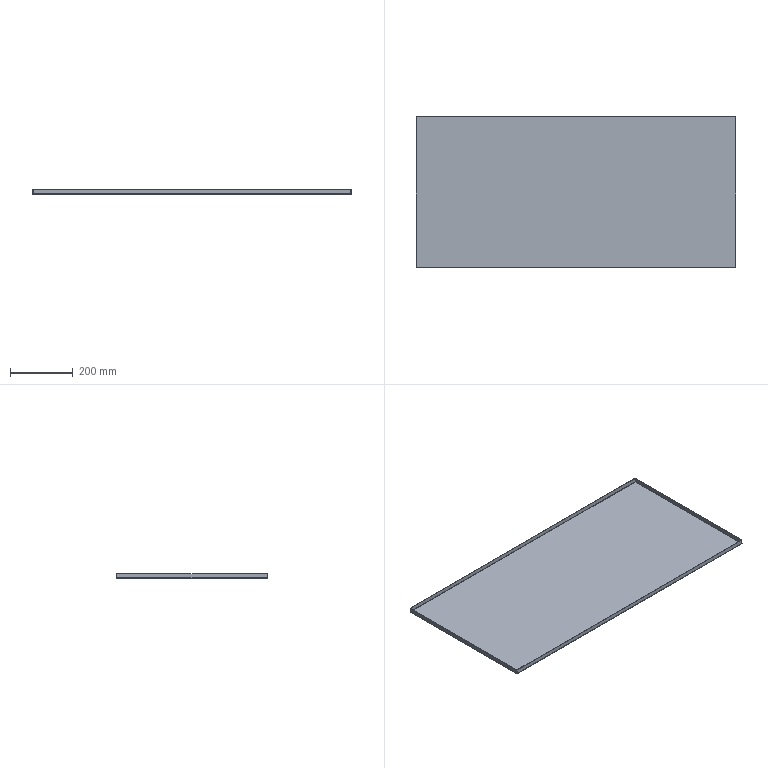Part | SolidWorks | 1 solid | 38 faces | box 1020 x 485.001 x 15 mm | volume 800985 mm3 | plane 22 | spline 8 | cylinder 8 | commonest cylinder face diameters 0.2 x4 3.2 x4
STEP:
#1=CARTESIAN_POINT('',(508.4,-240.9,-1.5));
#2=VERTEX_POINT('',#1);
#3=CARTESIAN_POINT('',(-508.4,-240.9,-1.5));
#4=VERTEX_POINT('',#3);
#5=CARTESIAN_POINT('',(508.4,-240.9,-1.5));
#6=DIRECTION('',(-1.,0.,0.));
#7=VECTOR('',#6,1000.);
#8=LINE('',#5,#7);
#9=EDGE_CURVE('',#2,#4,#8,.T.);
#10=ORIENTED_EDGE('',*,*,#9,.T.);
#11=CARTESIAN_POINT('',(-508.4,240.9,-1.5));
#12=VERTEX_POINT('',#11);
#13=CARTESIAN_POINT('',(-508.4,-240.9,-1.5));
#14=DIRECTION('',(0.,1.,0.));
#15=VECTOR('',#14,1000.);
#16=LINE('',#13,#15);
#17=EDGE_CURVE('',#4,#12,#16,.T.);
#18=ORIENTED_EDGE('',*,*,#17,.T.);
#19=CARTESIAN_POINT('',(508.4,240.9,-1.5));
#20=VERTEX_POINT('',#19);
#21=CARTESIAN_POINT('',(-508.4,240.9,-1.5));
#22=DIRECTION('',(1.,0.,0.));
#23=VECTOR('',#22,1000.);
#24=LINE('',#21,#23);
#25=EDGE_CURVE('',#12,#20,#24,.T.);
#26=ORIENTED_EDGE('',*,*,#25,.T.);
#27=CARTESIAN_POINT('',(508.4,240.9,-1.5));
#28=DIRECTION('',(0.,-1.,0.));
#29=VECTOR('',#28,1000.);
#30=LINE('',#27,#29);
#31=EDGE_CURVE('',#20,#2,#30,.T.);
#32=ORIENTED_EDGE('',*,*,#31,.T.);
#33=EDGE_LOOP('',(#10,#18,#26,#32));
#34=FACE_OUTER_BOUND('',#33,.T.);
#35=CARTESIAN_POINT('',(0.,0.,-1.5));
#36=DIRECTION('',(0.,0.,1.));
#37=DIRECTION('',(1.,0.,0.));
#38=AXIS2_PLACEMENT_3D('',#35,#36,#37);
#39=PLANE('',#38);
#40=ADVANCED_FACE('',(#34),#39,.F.);
#41=CARTESIAN_POINT('',(-508.4,-240.9,0.));
#42=VERTEX_POINT('',#41);
#43=CARTESIAN_POINT('',(-508.4,240.9,0.));
#44=VERTEX_POINT('',#43);
#45=CARTESIAN_POINT('',(-508.4,-240.9,0.));
#46=DIRECTION('',(0.,1.,0.));
#47=VECTOR('',#46,1000.);
#48=LINE('',#45,#47);
#49=EDGE_CURVE('',#42,#44,#48,.T.);
#50=ORIENTED_EDGE('',*,*,#49,.F.);
#51=CARTESIAN_POINT('',(508.4,-240.9,0.));
#52=VERTEX_POINT('',#51);
#53=CARTESIAN_POINT('',(508.4,-240.9,0.));
#54=DIRECTION('',(-1.,0.,0.));
#55=VECTOR('',#54,1000.);
#56=LINE('',#53,#55);
#57=EDGE_CURVE('',#52,#42,#56,.T.);
#58=ORIENTED_EDGE('',*,*,#57,.F.);
#59=CARTESIAN_POINT('',(508.4,240.9,0.));
#60=VERTEX_POINT('',#59);
#61=CARTESIAN_POINT('',(508.4,240.9,0.));
#62=DIRECTION('',(0.,-1.,0.));
#63=VECTOR('',#62,1000.);
#64=LINE('',#61,#63);
#65=EDGE_CURVE('',#60,#52,#64,.T.);
#66=ORIENTED_EDGE('',*,*,#65,.F.);
#67=CARTESIAN_POINT('',(-508.4,240.9,0.));
#68=DIRECTION('',(1.,0.,0.));
#69=VECTOR('',#68,1000.);
#70=LINE('',#67,#69);
#71=EDGE_CURVE('',#44,#60,#70,.T.);
#72=ORIENTED_EDGE('',*,*,#71,.F.);
#73=EDGE_LOOP('',(#50,#58,#66,#72));
#74=FACE_OUTER_BOUND('',#73,.T.);
#75=CARTESIAN_POINT('',(0.,0.,0.));
#76=DIRECTION('',(0.,0.,1.));
#77=DIRECTION('',(1.,0.,0.));
#78=AXIS2_PLACEMENT_3D('',#75,#76,#77);
#79=PLANE('',#78);
#80=ADVANCED_FACE('',(#74),#79,.T.);
#81=CARTESIAN_POINT('',(-510.,240.293,0.1));
#82=VERTEX_POINT('',#81);
#83=CARTESIAN_POINT('',(-508.5,240.293,0.1));
#84=VERTEX_POINT('',#83);
#85=CARTESIAN_POINT('',(-508.5,240.293,0.1));
#86=DIRECTION('',(1.,0.,0.));
#87=VECTOR('',#86,1000.);
#88=LINE('',#85,#87);
#89=EDGE_CURVE('',#82,#84,#88,.T.);
#90=ORIENTED_EDGE('',*,*,#89,.T.);
#91=CARTESIAN_POINT('',(-508.4,240.9,0.));
#92=CARTESIAN_POINT('',(-508.426,240.799,0.));
#93=CARTESIAN_POINT('',(-508.452,240.698,0.01078));
#94=CARTESIAN_POINT('',(-508.489,240.495,0.0478));
#95=CARTESIAN_POINT('',(-508.5,240.394,0.07382));
#96=CARTESIAN_POINT('',(-508.5,240.293,0.1));
#97=B_SPLINE_CURVE_WITH_KNOTS('',3,(#91,#92,#93,#94,#95,#96),.UNSPECIFIED.,.F.,.F.,(4,2,4),(0.,0.5,1.),.UNSPECIFIED.);
#98=EDGE_CURVE('',#44,#84,#97,.T.);
#99=ORIENTED_EDGE('',*,*,#98,.F.);
#100=CARTESIAN_POINT('',(-508.4,240.9,0.));
#101=DIRECTION('',(0.,0.,-1.));
#102=VECTOR('',#101,1000.);
#103=LINE('',#100,#102);
#104=EDGE_CURVE('',#44,#12,#103,.T.);
#105=ORIENTED_EDGE('',*,*,#104,.T.);
#106=CARTESIAN_POINT('',(-508.4,240.9,-1.5));
#107=CARTESIAN_POINT('',(-508.612,240.849,-1.5));
#108=CARTESIAN_POINT('',(-508.815,240.8,-1.46));
#109=CARTESIAN_POINT('',(-509.205,240.698,-1.299));
#110=CARTESIAN_POINT('',(-509.381,240.648,-1.181));
#111=CARTESIAN_POINT('',(-509.605,240.571,-0.9582));
#112=CARTESIAN_POINT('',(-509.671,240.546,-0.8775));
#113=CARTESIAN_POINT('',(-509.787,240.496,-0.7041));
#114=CARTESIAN_POINT('',(-509.838,240.47,-0.6103));
#115=CARTESIAN_POINT('',(-509.958,240.394,-0.32));
#116=CARTESIAN_POINT('',(-510.,240.344,-0.1115));
#117=CARTESIAN_POINT('',(-510.,240.293,0.1));
#118=B_SPLINE_CURVE_WITH_KNOTS('',3,(#106,#107,#108,#109,#110,#111,#112,#113,#114,#115,#116,#117),.UNSPECIFIED.,.F.,.F.,(4,2,2,2,2,4),(0.,0.0006399,0.00128,0.0016,0.00192,0.00256),.UNSPECIFIED.);
#119=EDGE_CURVE('',#12,#82,#118,.T.);
#120=ORIENTED_EDGE('',*,*,#119,.T.);
#121=EDGE_LOOP('',(#90,#99,#105,#120));
#122=FACE_OUTER_BOUND('',#121,.T.);
#123=CARTESIAN_POINT('',(-508.4,240.9,-1.515));
#124=CARTESIAN_POINT('',(-508.611,240.849,-1.515));
#125=CARTESIAN_POINT('',(-508.823,240.799,-1.473));
#126=CARTESIAN_POINT('',(-509.213,240.698,-1.311));
#127=CARTESIAN_POINT('',(-509.392,240.647,-1.191));
#128=CARTESIAN_POINT('',(-509.691,240.546,-0.8925));
#129=CARTESIAN_POINT('',(-509.811,240.495,-0.7133));
#130=CARTESIAN_POINT('',(-509.973,240.394,-0.3227));
#131=CARTESIAN_POINT('',(-510.015,240.343,-0.1114));
#132=CARTESIAN_POINT('',(-510.015,240.293,0.1));
#133=CARTESIAN_POINT('',(-508.4,240.9,-1.5));
#134=CARTESIAN_POINT('',(-508.609,240.849,-1.5));
#135=CARTESIAN_POINT('',(-508.819,240.799,-1.458));
#136=CARTESIAN_POINT('',(-509.206,240.698,-1.298));
#137=CARTESIAN_POINT('',(-509.383,240.647,-1.179));
#138=CARTESIAN_POINT('',(-509.679,240.546,-0.8833));
#139=CARTESIAN_POINT('',(-509.798,240.495,-0.7058));
#140=CARTESIAN_POINT('',(-509.958,240.394,-0.3188));
#141=CARTESIAN_POINT('',(-510.,240.343,-0.1095));
#142=CARTESIAN_POINT('',(-510.,240.293,0.1));
#143=CARTESIAN_POINT('',(-508.4,240.9,0.));
#144=CARTESIAN_POINT('',(-508.413,240.849,0.));
#145=CARTESIAN_POINT('',(-508.426,240.799,0.002603));
#146=CARTESIAN_POINT('',(-508.45,240.698,0.01262));
#147=CARTESIAN_POINT('',(-508.461,240.647,0.02003));
#148=CARTESIAN_POINT('',(-508.48,240.546,0.03855));
#149=CARTESIAN_POINT('',(-508.487,240.495,0.04964));
#150=CARTESIAN_POINT('',(-508.497,240.394,0.07383));
#151=CARTESIAN_POINT('',(-508.5,240.343,0.08691));
#152=CARTESIAN_POINT('',(-508.5,240.293,0.1));
#153=B_SPLINE_SURFACE_WITH_KNOTS('',1,3,((#123,#124,#125,#126,#127,#128,#129,#130,#131,#132),(#133,#134,#135,#136,#137,#138,#139,#140,#141,#142),(#143,#144,#145,#146,#147,#148,#149,#150,#151,#152)),.UNSPECIFIED.,.F.,.F.,.F.,(2,1,2),(4,2,2,2,4),(-0.01,0.,1.),(0.,0.25,0.5,0.75,1.),.UNSPECIFIED.);
#154=ADVANCED_FACE('',(#122),#153,.F.);
#155=CARTESIAN_POINT('',(-508.5,-240.293,0.1));
#156=VERTEX_POINT('',#155);
#157=CARTESIAN_POINT('',(-508.5,-240.293,0.1));
#158=CARTESIAN_POINT('',(-508.5,-240.394,0.07382));
#159=CARTESIAN_POINT('',(-508.489,-240.495,0.0478));
#160=CARTESIAN_POINT('',(-508.452,-240.698,0.01078));
#161=CARTESIAN_POINT('',(-508.426,-240.799,0.));
#162=CARTESIAN_POINT('',(-508.4,-240.9,0.));
#163=B_SPLINE_CURVE_WITH_KNOTS('',3,(#157,#158,#159,#160,#161,#162),.UNSPECIFIED.,.F.,.F.,(4,2,4),(0.,0.5,1.),.UNSPECIFIED.);
#164=EDGE_CURVE('',#156,#42,#163,.T.);
#165=ORIENTED_EDGE('',*,*,#164,.F.);
#166=CARTESIAN_POINT('',(-510.,-240.293,0.1));
#167=VERTEX_POINT('',#166);
#168=CARTESIAN_POINT('',(-508.5,-240.293,0.1));
#169=DIRECTION('',(1.,0.,0.));
#170=VECTOR('',#169,1000.);
#171=LINE('',#168,#170);
#172=EDGE_CURVE('',#167,#156,#171,.T.);
#173=ORIENTED_EDGE('',*,*,#172,.F.);
#174=CARTESIAN_POINT('',(-510.,-240.293,0.1));
#175=CARTESIAN_POINT('',(-510.,-240.344,-0.1115));
#176=CARTESIAN_POINT('',(-509.96,-240.393,-0.3151));
#177=CARTESIAN_POINT('',(-509.799,-240.495,-0.7048));
#178=CARTESIAN_POINT('',(-509.681,-240.545,-0.881));
#179=CARTESIAN_POINT('',(-509.458,-240.621,-1.105));
#180=CARTESIAN_POINT('',(-509.378,-240.647,-1.171));
#181=CARTESIAN_POINT('',(-509.204,-240.697,-1.287));
#182=CARTESIAN_POINT('',(-509.11,-240.723,-1.338));
#183=CARTESIAN_POINT('',(-508.82,-240.799,-1.458));
#184=CARTESIAN_POINT('',(-508.612,-240.849,-1.5));
#185=CARTESIAN_POINT('',(-508.4,-240.9,-1.5));
#186=B_SPLINE_CURVE_WITH_KNOTS('',3,(#174,#175,#176,#177,#178,#179,#180,#181,#182,#183,#184,#185),.UNSPECIFIED.,.F.,.F.,(4,2,2,2,2,4),(0.,0.0006399,0.00128,0.0016,0.00192,0.00256),.UNSPECIFIED.);
#187=EDGE_CURVE('',#167,#4,#186,.T.);
#188=ORIENTED_EDGE('',*,*,#187,.T.);
#189=CARTESIAN_POINT('',(-508.4,-240.9,0.));
#190=DIRECTION('',(0.,0.,-1.));
#191=VECTOR('',#190,1000.);
#192=LINE('',#189,#191);
#193=EDGE_CURVE('',#42,#4,#192,.T.);
#194=ORIENTED_EDGE('',*,*,#193,.F.);
#195=EDGE_LOOP('',(#165,#173,#188,#194));
#196=FACE_OUTER_BOUND('',#195,.T.);
#197=CARTESIAN_POINT('',(-510.015,-240.293,0.1));
#198=CARTESIAN_POINT('',(-510.015,-240.343,-0.1114));
#199=CARTESIAN_POINT('',(-509.973,-240.394,-0.3227));
#200=CARTESIAN_POINT('',(-509.811,-240.495,-0.7133));
#201=CARTESIAN_POINT('',(-509.691,-240.546,-0.8925));
#202=CARTESIAN_POINT('',(-509.392,-240.647,-1.191));
#203=CARTESIAN_POINT('',(-509.213,-240.698,-1.311));
#204=CARTESIAN_POINT('',(-508.823,-240.799,-1.473));
#205=CARTESIAN_POINT('',(-508.611,-240.849,-1.515));
#206=CARTESIAN_POINT('',(-508.4,-240.9,-1.515));
#207=CARTESIAN_POINT('',(-510.,-240.293,0.1));
#208=CARTESIAN_POINT('',(-510.,-240.343,-0.1095));
#209=CARTESIAN_POINT('',(-509.958,-240.394,-0.3188));
#210=CARTESIAN_POINT('',(-509.798,-240.495,-0.7058));
#211=CARTESIAN_POINT('',(-509.679,-240.546,-0.8833));
#212=CARTESIAN_POINT('',(-509.383,-240.647,-1.179));
#213=CARTESIAN_POINT('',(-509.206,-240.698,-1.298));
#214=CARTESIAN_POINT('',(-508.819,-240.799,-1.458));
#215=CARTESIAN_POINT('',(-508.609,-240.849,-1.5));
#216=CARTESIAN_POINT('',(-508.4,-240.9,-1.5));
#217=CARTESIAN_POINT('',(-508.5,-240.293,0.1));
#218=CARTESIAN_POINT('',(-508.5,-240.343,0.08691));
#219=CARTESIAN_POINT('',(-508.497,-240.394,0.07383));
#220=CARTESIAN_POINT('',(-508.487,-240.495,0.04964));
#221=CARTESIAN_POINT('',(-508.48,-240.546,0.03855));
#222=CARTESIAN_POINT('',(-508.461,-240.647,0.02003));
#223=CARTESIAN_POINT('',(-508.45,-240.698,0.01262));
#224=CARTESIAN_POINT('',(-508.426,-240.799,0.002603));
#225=CARTESIAN_POINT('',(-508.413,-240.849,0.));
#226=CARTESIAN_POINT('',(-508.4,-240.9,0.));
#227=B_SPLINE_SURFACE_WITH_KNOTS('',1,3,((#197,#198,#199,#200,#201,#202,#203,#204,#205,#206),(#207,#208,#209,#210,#211,#212,#213,#214,#215,#216),(#217,#218,#219,#220,#221,#222,#223,#224,#225,#226)),.UNSPECIFIED.,.F.,.F.,.F.,(2,1,2),(4,2,2,2,4),(-0.01,0.,1.),(0.,0.25,0.5,0.75,1.),.UNSPECIFIED.);
#228=ADVANCED_FACE('',(#196),#227,.F.);
#229=ORIENTED_EDGE('',*,*,#17,.F.);
#230=ORIENTED_EDGE('',*,*,#187,.F.);
#231=CARTESIAN_POINT('',(-510.,242.5,0.1));
#232=DIRECTION('',(0.,1.,0.));
#233=VECTOR('',#232,1000.);
#234=LINE('',#231,#233);
#235=EDGE_CURVE('',#167,#82,#234,.T.);
#236=ORIENTED_EDGE('',*,*,#235,.T.);
#237=ORIENTED_EDGE('',*,*,#119,.F.);
#238=EDGE_LOOP('',(#229,#230,#236,#237));
#239=FACE_OUTER_BOUND('',#238,.T.);
#240=CARTESIAN_POINT('',(-508.4,-240.9,0.1));
#241=DIRECTION('',(0.,-1.,0.));
#242=DIRECTION('',(-1.,0.,0.));
#243=AXIS2_PLACEMENT_3D('',#240,#241,#242);
#244=CYLINDRICAL_SURFACE('',#243,1.6);
#245=ADVANCED_FACE('',(#239),#244,.T.);
#246=ORIENTED_EDGE('',*,*,#49,.T.);
#247=ORIENTED_EDGE('',*,*,#98,.T.);
#248=CARTESIAN_POINT('',(-508.5,242.5,0.1));
#249=DIRECTION('',(0.,-1.,0.));
#250=VECTOR('',#249,1000.);
#251=LINE('',#248,#250);
#252=EDGE_CURVE('',#84,#156,#251,.T.);
#253=ORIENTED_EDGE('',*,*,#252,.T.);
#254=ORIENTED_EDGE('',*,*,#164,.T.);
#255=EDGE_LOOP('',(#246,#247,#253,#254));
#256=FACE_OUTER_BOUND('',#255,.T.);
#257=CARTESIAN_POINT('',(-508.4,-240.9,0.1));
#258=DIRECTION('',(0.,-1.,0.));
#259=DIRECTION('',(-1.,0.,0.));
#260=AXIS2_PLACEMENT_3D('',#257,#258,#259);
#261=CYLINDRICAL_SURFACE('',#260,0.1);
#262=ADVANCED_FACE('',(#256),#261,.F.);
#263=CARTESIAN_POINT('',(-510.,240.293,13.5));
#264=VERTEX_POINT('',#263);
#265=CARTESIAN_POINT('',(-510.,240.293,0.));
#266=DIRECTION('',(0.,0.,1.));
#267=VECTOR('',#266,1000.);
#268=LINE('',#265,#267);
#269=EDGE_CURVE('',#82,#264,#268,.T.);
#270=ORIENTED_EDGE('',*,*,#269,.T.);
#271=CARTESIAN_POINT('',(-508.5,240.293,13.5));
#272=VERTEX_POINT('',#271);
#273=CARTESIAN_POINT('',(-508.5,240.293,13.5));
#274=DIRECTION('',(1.,0.,0.));
#275=VECTOR('',#274,1000.);
#276=LINE('',#273,#275);
#277=EDGE_CURVE('',#264,#272,#276,.T.);
#278=ORIENTED_EDGE('',*,*,#277,.T.);
#279=CARTESIAN_POINT('',(-508.5,240.293,0.));
#280=DIRECTION('',(0.,0.,1.));
#281=VECTOR('',#280,1000.);
#282=LINE('',#279,#281);
#283=EDGE_CURVE('',#84,#272,#282,.T.);
#284=ORIENTED_EDGE('',*,*,#283,.F.);
#285=ORIENTED_EDGE('',*,*,#89,.F.);
#286=EDGE_LOOP('',(#270,#278,#284,#285));
#287=FACE_OUTER_BOUND('',#286,.T.);
#288=CARTESIAN_POINT('',(-508.5,240.293,0.));
#289=DIRECTION('',(0.,1.,0.));
#290=DIRECTION('',(0.,0.,1.));
#291=AXIS2_PLACEMENT_3D('',#288,#289,#290);
#292=PLANE('',#291);
#293=ADVANCED_FACE('',(#287),#292,.T.);
#294=ORIENTED_EDGE('',*,*,#235,.F.);
#295=CARTESIAN_POINT('',(-510.,-240.293,13.5));
#296=VERTEX_POINT('',#295);
#297=CARTESIAN_POINT('',(-510.,-240.293,0.));
#298=DIRECTION('',(0.,0.,1.));
#299=VECTOR('',#298,1000.);
#300=LINE('',#297,#299);
#301=EDGE_CURVE('',#167,#296,#300,.T.);
#302=ORIENTED_EDGE('',*,*,#301,.T.);
#303=CARTESIAN_POINT('',(-510.,0.,13.5));
#304=DIRECTION('',(0.,1.,0.));
#305=VECTOR('',#304,1000.);
#306=LINE('',#303,#305);
#307=EDGE_CURVE('',#296,#264,#306,.T.);
#308=ORIENTED_EDGE('',*,*,#307,.T.);
#309=ORIENTED_EDGE('',*,*,#269,.F.);
#310=EDGE_LOOP('',(#294,#302,#308,#309));
#311=FACE_OUTER_BOUND('',#310,.T.);
#312=CARTESIAN_POINT('',(-510.,0.,0.));
#313=DIRECTION('',(1.,0.,0.));
#314=DIRECTION('',(0.,0.,-1.));
#315=AXIS2_PLACEMENT_3D('',#312,#313,#314);
#316=PLANE('',#315);
#317=ADVANCED_FACE('',(#311),#316,.F.);
#318=CARTESIAN_POINT('',(-508.5,-240.293,13.5));
#319=VERTEX_POINT('',#318);
#320=CARTESIAN_POINT('',(-508.5,-240.293,0.));
#321=DIRECTION('',(0.,0.,1.));
#322=VECTOR('',#321,1000.);
#323=LINE('',#320,#322);
#324=EDGE_CURVE('',#156,#319,#323,.T.);
#325=ORIENTED_EDGE('',*,*,#324,.F.);
#326=ORIENTED_EDGE('',*,*,#252,.F.);
#327=ORIENTED_EDGE('',*,*,#283,.T.);
#328=CARTESIAN_POINT('',(-508.5,242.5,13.5));
#329=DIRECTION('',(0.,1.,0.));
#330=VECTOR('',#329,1000.);
#331=LINE('',#328,#330);
#332=EDGE_CURVE('',#319,#272,#331,.T.);
#333=ORIENTED_EDGE('',*,*,#332,.F.);
#334=EDGE_LOOP('',(#325,#326,#327,#333));
#335=FACE_OUTER_BOUND('',#334,.T.);
#336=CARTESIAN_POINT('',(-508.5,0.,0.));
#337=DIRECTION('',(1.,0.,0.));
#338=DIRECTION('',(0.,0.,-1.));
#339=AXIS2_PLACEMENT_3D('',#336,#337,#338);
#340=PLANE('',#339);
#341=ADVANCED_FACE('',(#335),#340,.T.);
#342=ORIENTED_EDGE('',*,*,#307,.F.);
#343=CARTESIAN_POINT('',(-510.,-240.293,13.5));
#344=DIRECTION('',(1.,0.,0.));
#345=VECTOR('',#344,1000.);
#346=LINE('',#343,#345);
#347=EDGE_CURVE('',#296,#319,#346,.T.);
#348=ORIENTED_EDGE('',*,*,#347,.T.);
#349=ORIENTED_EDGE('',*,*,#332,.T.);
#350=ORIENTED_EDGE('',*,*,#277,.F.);
#351=EDGE_LOOP('',(#342,#348,#349,#350));
#352=FACE_OUTER_BOUND('',#351,.T.);
#353=CARTESIAN_POINT('',(-510.,242.5,13.5));
#354=DIRECTION('',(0.,0.,-1.));
#355=DIRECTION('',(-1.,0.,0.));
#356=AXIS2_PLACEMENT_3D('',#353,#354,#355);
#357=PLANE('',#356);
#358=ADVANCED_FACE('',(#352),#357,.F.);
#359=ORIENTED_EDGE('',*,*,#347,.F.);
#360=ORIENTED_EDGE('',*,*,#301,.F.);
#361=ORIENTED_EDGE('',*,*,#172,.T.);
#362=ORIENTED_EDGE('',*,*,#324,.T.);
#363=EDGE_LOOP('',(#359,#360,#361,#362));
#364=FACE_OUTER_BOUND('',#363,.T.);
#365=CARTESIAN_POINT('',(-508.5,-240.293,0.));
#366=DIRECTION('',(0.,1.,0.));
#367=DIRECTION('',(0.,0.,1.));
#368=AXIS2_PLACEMENT_3D('',#365,#366,#367);
#369=PLANE('',#368);
#370=ADVANCED_FACE('',(#364),#369,.F.);
#371=CARTESIAN_POINT('',(507.793,242.5,0.1));
#372=VERTEX_POINT('',#371);
#373=CARTESIAN_POINT('',(507.793,241.,0.1));
#374=VERTEX_POINT('',#373);
#375=CARTESIAN_POINT('',(507.793,241.,0.1));
#376=DIRECTION('',(0.,-1.,0.));
#377=VECTOR('',#376,1000.);
#378=LINE('',#375,#377);
#379=EDGE_CURVE('',#372,#374,#378,.T.);
#380=ORIENTED_EDGE('',*,*,#379,.T.);
#381=CARTESIAN_POINT('',(508.4,240.9,0.));
#382=CARTESIAN_POINT('',(508.299,240.926,0.));
#383=CARTESIAN_POINT('',(508.198,240.952,0.01078));
#384=CARTESIAN_POINT('',(507.995,240.989,0.0478));
#385=CARTESIAN_POINT('',(507.894,241.,0.07382));
#386=CARTESIAN_POINT('',(507.793,241.,0.1));
#387=B_SPLINE_CURVE_WITH_KNOTS('',3,(#381,#382,#383,#384,#385,#386),.UNSPECIFIED.,.F.,.F.,(4,2,4),(0.,0.5,1.),.UNSPECIFIED.);
#388=EDGE_CURVE('',#60,#374,#387,.T.);
#389=ORIENTED_EDGE('',*,*,#388,.F.);
#390=CARTESIAN_POINT('',(508.4,240.9,0.));
#391=DIRECTION('',(0.,0.,-1.));
#392=VECTOR('',#391,1000.);
#393=LINE('',#390,#392);
#394=EDGE_CURVE('',#60,#20,#393,.T.);
#395=ORIENTED_EDGE('',*,*,#394,.T.);
#396=CARTESIAN_POINT('',(508.4,240.9,-1.5));
#397=CARTESIAN_POINT('',(508.349,241.112,-1.5));
#398=CARTESIAN_POINT('',(508.3,241.315,-1.46));
#399=CARTESIAN_POINT('',(508.198,241.705,-1.299));
#400=CARTESIAN_POINT('',(508.148,241.881,-1.181));
#401=CARTESIAN_POINT('',(508.071,242.105,-0.9582));
#402=CARTESIAN_POINT('',(508.046,242.171,-0.8775));
#403=CARTESIAN_POINT('',(507.996,242.287,-0.7041));
#404=CARTESIAN_POINT('',(507.97,242.338,-0.6103));
#405=CARTESIAN_POINT('',(507.894,242.458,-0.32));
#406=CARTESIAN_POINT('',(507.844,242.5,-0.1115));
#407=CARTESIAN_POINT('',(507.793,242.5,0.1));
#408=B_SPLINE_CURVE_WITH_KNOTS('',3,(#396,#397,#398,#399,#400,#401,#402,#403,#404,#405,#406,#407),.UNSPECIFIED.,.F.,.F.,(4,2,2,2,2,4),(0.,0.0006399,0.00128,0.0016,0.00192,0.00256),.UNSPECIFIED.);
#409=EDGE_CURVE('',#20,#372,#408,.T.);
#410=ORIENTED_EDGE('',*,*,#409,.T.);
#411=EDGE_LOOP('',(#380,#389,#395,#410));
#412=FACE_OUTER_BOUND('',#411,.T.);
#413=CARTESIAN_POINT('',(508.4,240.9,-1.515));
#414=CARTESIAN_POINT('',(508.349,241.111,-1.515));
#415=CARTESIAN_POINT('',(508.299,241.323,-1.473));
#416=CARTESIAN_POINT('',(508.198,241.713,-1.311));
#417=CARTESIAN_POINT('',(508.147,241.892,-1.191));
#418=CARTESIAN_POINT('',(508.046,242.191,-0.8925));
#419=CARTESIAN_POINT('',(507.995,242.311,-0.7133));
#420=CARTESIAN_POINT('',(507.894,242.473,-0.3227));
#421=CARTESIAN_POINT('',(507.843,242.515,-0.1114));
#422=CARTESIAN_POINT('',(507.793,242.515,0.1));
#423=CARTESIAN_POINT('',(508.4,240.9,-1.5));
#424=CARTESIAN_POINT('',(508.349,241.109,-1.5));
#425=CARTESIAN_POINT('',(508.299,241.319,-1.458));
#426=CARTESIAN_POINT('',(508.198,241.706,-1.298));
#427=CARTESIAN_POINT('',(508.147,241.883,-1.179));
#428=CARTESIAN_POINT('',(508.046,242.179,-0.8833));
#429=CARTESIAN_POINT('',(507.995,242.298,-0.7058));
#430=CARTESIAN_POINT('',(507.894,242.458,-0.3188));
#431=CARTESIAN_POINT('',(507.843,242.5,-0.1095));
#432=CARTESIAN_POINT('',(507.793,242.5,0.1));
#433=CARTESIAN_POINT('',(508.4,240.9,0.));
#434=CARTESIAN_POINT('',(508.349,240.913,0.));
#435=CARTESIAN_POINT('',(508.299,240.926,0.002603));
#436=CARTESIAN_POINT('',(508.198,240.95,0.01262));
#437=CARTESIAN_POINT('',(508.147,240.961,0.02003));
#438=CARTESIAN_POINT('',(508.046,240.98,0.03855));
#439=CARTESIAN_POINT('',(507.995,240.987,0.04964));
#440=CARTESIAN_POINT('',(507.894,240.997,0.07383));
#441=CARTESIAN_POINT('',(507.843,241.,0.08691));
#442=CARTESIAN_POINT('',(507.793,241.,0.1));
#443=B_SPLINE_SURFACE_WITH_KNOTS('',1,3,((#413,#414,#415,#416,#417,#418,#419,#420,#421,#422),(#423,#424,#425,#426,#427,#428,#429,#430,#431,#432),(#433,#434,#435,#436,#437,#438,#439,#440,#441,#442)),.UNSPECIFIED.,.F.,.F.,.F.,(2,1,2),(4,2,2,2,4),(-0.01,0.,1.),(0.,0.25,0.5,0.75,1.),.UNSPECIFIED.);
#444=ADVANCED_FACE('',(#412),#443,.F.);
#445=CARTESIAN_POINT('',(-507.793,241.,0.1));
#446=VERTEX_POINT('',#445);
#447=CARTESIAN_POINT('',(-507.793,241.,0.1));
#448=CARTESIAN_POINT('',(-507.894,241.,0.07382));
#449=CARTESIAN_POINT('',(-507.995,240.989,0.0478));
#450=CARTESIAN_POINT('',(-508.198,240.952,0.01078));
#451=CARTESIAN_POINT('',(-508.299,240.926,0.));
#452=CARTESIAN_POINT('',(-508.4,240.9,0.));
#453=B_SPLINE_CURVE_WITH_KNOTS('',3,(#447,#448,#449,#450,#451,#452),.UNSPECIFIED.,.F.,.F.,(4,2,4),(0.,0.5,1.),.UNSPECIFIED.);
#454=EDGE_CURVE('',#446,#44,#453,.T.);
#455=ORIENTED_EDGE('',*,*,#454,.F.);
#456=CARTESIAN_POINT('',(-507.793,242.5,0.1));
#457=VERTEX_POINT('',#456);
#458=CARTESIAN_POINT('',(-507.793,241.,0.1));
#459=DIRECTION('',(0.,-1.,0.));
#460=VECTOR('',#459,1000.);
#461=LINE('',#458,#460);
#462=EDGE_CURVE('',#457,#446,#461,.T.);
#463=ORIENTED_EDGE('',*,*,#462,.F.);
#464=CARTESIAN_POINT('',(-507.793,242.5,0.1));
#465=CARTESIAN_POINT('',(-507.844,242.5,-0.1115));
#466=CARTESIAN_POINT('',(-507.893,242.46,-0.3151));
#467=CARTESIAN_POINT('',(-507.995,242.299,-0.7048));
#468=CARTESIAN_POINT('',(-508.045,242.181,-0.881));
#469=CARTESIAN_POINT('',(-508.121,241.958,-1.105));
#470=CARTESIAN_POINT('',(-508.147,241.878,-1.171));
#471=CARTESIAN_POINT('',(-508.197,241.704,-1.287));
#472=CARTESIAN_POINT('',(-508.223,241.61,-1.338));
#473=CARTESIAN_POINT('',(-508.299,241.32,-1.458));
#474=CARTESIAN_POINT('',(-508.349,241.112,-1.5));
#475=CARTESIAN_POINT('',(-508.4,240.9,-1.5));
#476=B_SPLINE_CURVE_WITH_KNOTS('',3,(#464,#465,#466,#467,#468,#469,#470,#471,#472,#473,#474,#475),.UNSPECIFIED.,.F.,.F.,(4,2,2,2,2,4),(0.,0.0006399,0.00128,0.0016,0.00192,0.00256),.UNSPECIFIED.);
#477=EDGE_CURVE('',#457,#12,#476,.T.);
#478=ORIENTED_EDGE('',*,*,#477,.T.);
#479=ORIENTED_EDGE('',*,*,#104,.F.);
#480=EDGE_LOOP('',(#455,#463,#478,#479));
#481=FACE_OUTER_BOUND('',#480,.T.);
#482=CARTESIAN_POINT('',(-507.793,242.515,0.1));
#483=CARTESIAN_POINT('',(-507.843,242.515,-0.1114));
#484=CARTESIAN_POINT('',(-507.894,242.473,-0.3227));
#485=CARTESIAN_POINT('',(-507.995,242.311,-0.7133));
#486=CARTESIAN_POINT('',(-508.046,242.191,-0.8925));
#487=CARTESIAN_POINT('',(-508.147,241.892,-1.191));
#488=CARTESIAN_POINT('',(-508.198,241.713,-1.311));
#489=CARTESIAN_POINT('',(-508.299,241.323,-1.473));
#490=CARTESIAN_POINT('',(-508.349,241.111,-1.515));
#491=CARTESIAN_POINT('',(-508.4,240.9,-1.515));
#492=CARTESIAN_POINT('',(-507.793,242.5,0.1));
#493=CARTESIAN_POINT('',(-507.843,242.5,-0.1095));
#494=CARTESIAN_POINT('',(-507.894,242.458,-0.3188));
#495=CARTESIAN_POINT('',(-507.995,242.298,-0.7058));
#496=CARTESIAN_POINT('',(-508.046,242.179,-0.8833));
#497=CARTESIAN_POINT('',(-508.147,241.883,-1.179));
#498=CARTESIAN_POINT('',(-508.198,241.706,-1.298));
#499=CARTESIAN_POINT('',(-508.299,241.319,-1.458));
#500=CARTESIAN_POINT('',(-508.349,241.109,-1.5));
#501=CARTESIAN_POINT('',(-508.4,240.9,-1.5));
#502=CARTESIAN_POINT('',(-507.793,241.,0.1));
#503=CARTESIAN_POINT('',(-507.843,241.,0.08691));
#504=CARTESIAN_POINT('',(-507.894,240.997,0.07383));
#505=CARTESIAN_POINT('',(-507.995,240.987,0.04964));
#506=CARTESIAN_POINT('',(-508.046,240.98,0.03855));
#507=CARTESIAN_POINT('',(-508.147,240.961,0.02003));
#508=CARTESIAN_POINT('',(-508.198,240.95,0.01262));
#509=CARTESIAN_POINT('',(-508.299,240.926,0.002603));
#510=CARTESIAN_POINT('',(-508.349,240.913,0.));
#511=CARTESIAN_POINT('',(-508.4,240.9,0.));
#512=B_SPLINE_SURFACE_WITH_KNOTS('',1,3,((#482,#483,#484,#485,#486,#487,#488,#489,#490,#491),(#492,#493,#494,#495,#496,#497,#498,#499,#500,#501),(#502,#503,#504,#505,#506,#507,#508,#509,#510,#511)),.UNSPECIFIED.,.F.,.F.,.F.,(2,1,2),(4,2,2,2,4),(-0.01,0.,1.),(0.,0.25,0.5,0.75,1.),.UNSPECIFIED.);
#513=ADVANCED_FACE('',(#481),#512,.F.);
#514=ORIENTED_EDGE('',*,*,#25,.F.);
#515=ORIENTED_EDGE('',*,*,#477,.F.);
#516=CARTESIAN_POINT('',(510.,242.5,0.1));
#517=DIRECTION('',(1.,0.,0.));
#518=VECTOR('',#517,1000.);
#519=LINE('',#516,#518);
#520=EDGE_CURVE('',#457,#372,#519,.T.);
#521=ORIENTED_EDGE('',*,*,#520,.T.);
#522=ORIENTED_EDGE('',*,*,#409,.F.);
#523=EDGE_LOOP('',(#514,#515,#521,#522));
#524=FACE_OUTER_BOUND('',#523,.T.);
#525=CARTESIAN_POINT('',(-508.4,240.9,0.1));
#526=DIRECTION('',(-1.,0.,0.));
#527=DIRECTION('',(0.,1.,0.));
#528=AXIS2_PLACEMENT_3D('',#525,#526,#527);
#529=CYLINDRICAL_SURFACE('',#528,1.6);
#530=ADVANCED_FACE('',(#524),#529,.T.);
#531=ORIENTED_EDGE('',*,*,#71,.T.);
#532=ORIENTED_EDGE('',*,*,#388,.T.);
#533=CARTESIAN_POINT('',(510.,241.,0.1));
#534=DIRECTION('',(-1.,0.,0.));
#535=VECTOR('',#534,1000.);
#536=LINE('',#533,#535);
#537=EDGE_CURVE('',#374,#446,#536,.T.);
#538=ORIENTED_EDGE('',*,*,#537,.T.);
#539=ORIENTED_EDGE('',*,*,#454,.T.);
#540=EDGE_LOOP('',(#531,#532,#538,#539));
#541=FACE_OUTER_BOUND('',#540,.T.);
#542=CARTESIAN_POINT('',(-508.4,240.9,0.1));
#543=DIRECTION('',(-1.,0.,0.));
#544=DIRECTION('',(0.,1.,0.));
#545=AXIS2_PLACEMENT_3D('',#542,#543,#544);
#546=CYLINDRICAL_SURFACE('',#545,0.1);
#547=ADVANCED_FACE('',(#541),#546,.F.);
#548=CARTESIAN_POINT('',(507.793,242.5,13.5));
#549=VERTEX_POINT('',#548);
#550=CARTESIAN_POINT('',(507.793,242.5,0.));
#551=DIRECTION('',(0.,0.,1.));
#552=VECTOR('',#551,1000.);
#553=LINE('',#550,#552);
#554=EDGE_CURVE('',#372,#549,#553,.T.);
#555=ORIENTED_EDGE('',*,*,#554,.T.);
#556=CARTESIAN_POINT('',(507.793,241.,13.5));
#557=VERTEX_POINT('',#556);
#558=CARTESIAN_POINT('',(507.793,241.,13.5));
#559=DIRECTION('',(0.,-1.,0.));
#560=VECTOR('',#559,1000.);
#561=LINE('',#558,#560);
#562=EDGE_CURVE('',#549,#557,#561,.T.);
#563=ORIENTED_EDGE('',*,*,#562,.T.);
#564=CARTESIAN_POINT('',(507.793,241.,0.));
#565=DIRECTION('',(0.,0.,1.));
#566=VECTOR('',#565,1000.);
#567=LINE('',#564,#566);
#568=EDGE_CURVE('',#374,#557,#567,.T.);
#569=ORIENTED_EDGE('',*,*,#568,.F.);
#570=ORIENTED_EDGE('',*,*,#379,.F.);
#571=EDGE_LOOP('',(#555,#563,#569,#570));
#572=FACE_OUTER_BOUND('',#571,.T.);
#573=CARTESIAN_POINT('',(507.793,241.,0.));
#574=DIRECTION('',(1.,0.,0.));
#575=DIRECTION('',(0.,0.,-1.));
#576=AXIS2_PLACEMENT_3D('',#573,#574,#575);
#577=PLANE('',#576);
#578=ADVANCED_FACE('',(#572),#577,.T.);
#579=ORIENTED_EDGE('',*,*,#520,.F.);
#580=CARTESIAN_POINT('',(-507.793,242.5,13.5));
#581=VERTEX_POINT('',#580);
#582=CARTESIAN_POINT('',(-507.793,242.5,0.));
#583=DIRECTION('',(0.,0.,1.));
#584=VECTOR('',#583,1000.);
#585=LINE('',#582,#584);
#586=EDGE_CURVE('',#457,#581,#585,.T.);
#587=ORIENTED_EDGE('',*,*,#586,.T.);
#588=CARTESIAN_POINT('',(0.,242.5,13.5));
#589=DIRECTION('',(1.,0.,0.));
#590=VECTOR('',#589,1000.);
#591=LINE('',#588,#590);
#592=EDGE_CURVE('',#581,#549,#591,.T.);
#593=ORIENTED_EDGE('',*,*,#592,.T.);
#594=ORIENTED_EDGE('',*,*,#554,.F.);
#595=EDGE_LOOP('',(#579,#587,#593,#594));
#596=FACE_OUTER_BOUND('',#595,.T.);
#597=CARTESIAN_POINT('',(0.,242.5,0.));
#598=DIRECTION('',(0.,-1.,0.));
#599=DIRECTION('',(0.,0.,-1.));
#600=AXIS2_PLACEMENT_3D('',#597,#598,#599);
#601=PLANE('',#600);
#602=ADVANCED_FACE('',(#596),#601,.F.);
#603=CARTESIAN_POINT('',(-507.793,241.,13.5));
#604=VERTEX_POINT('',#603);
#605=CARTESIAN_POINT('',(-507.793,241.,0.));
#606=DIRECTION('',(0.,0.,1.));
#607=VECTOR('',#606,1000.);
#608=LINE('',#605,#607);
#609=EDGE_CURVE('',#446,#604,#608,.T.);
#610=ORIENTED_EDGE('',*,*,#609,.F.);
#611=ORIENTED_EDGE('',*,*,#537,.F.);
#612=ORIENTED_EDGE('',*,*,#568,.T.);
#613=CARTESIAN_POINT('',(510.,241.,13.5));
#614=DIRECTION('',(1.,0.,0.));
#615=VECTOR('',#614,1000.);
#616=LINE('',#613,#615);
#617=EDGE_CURVE('',#604,#557,#616,.T.);
#618=ORIENTED_EDGE('',*,*,#617,.F.);
#619=EDGE_LOOP('',(#610,#611,#612,#618));
#620=FACE_OUTER_BOUND('',#619,.T.);
#621=CARTESIAN_POINT('',(0.,241.,0.));
#622=DIRECTION('',(0.,-1.,0.));
#623=DIRECTION('',(0.,0.,-1.));
#624=AXIS2_PLACEMENT_3D('',#621,#622,#623);
#625=PLANE('',#624);
#626=ADVANCED_FACE('',(#620),#625,.T.);
#627=ORIENTED_EDGE('',*,*,#592,.F.);
#628=CARTESIAN_POINT('',(-507.793,242.5,13.5));
#629=DIRECTION('',(0.,-1.,0.));
#630=VECTOR('',#629,1000.);
#631=LINE('',#628,#630);
#632=EDGE_CURVE('',#581,#604,#631,.T.);
#633=ORIENTED_EDGE('',*,*,#632,.T.);
#634=ORIENTED_EDGE('',*,*,#617,.T.);
#635=ORIENTED_EDGE('',*,*,#562,.F.);
#636=EDGE_LOOP('',(#627,#633,#634,#635));
#637=FACE_OUTER_BOUND('',#636,.T.);
#638=CARTESIAN_POINT('',(510.,242.5,13.5));
#639=DIRECTION('',(0.,0.,-1.));
#640=DIRECTION('',(0.,1.,0.));
#641=AXIS2_PLACEMENT_3D('',#638,#639,#640);
#642=PLANE('',#641);
#643=ADVANCED_FACE('',(#637),#642,.F.);
#644=ORIENTED_EDGE('',*,*,#632,.F.);
#645=ORIENTED_EDGE('',*,*,#586,.F.);
#646=ORIENTED_EDGE('',*,*,#462,.T.);
#647=ORIENTED_EDGE('',*,*,#609,.T.);
#648=EDGE_LOOP('',(#644,#645,#646,#647));
#649=FACE_OUTER_BOUND('',#648,.T.);
#650=CARTESIAN_POINT('',(-507.793,241.,0.));
#651=DIRECTION('',(1.,0.,0.));
#652=DIRECTION('',(0.,0.,-1.));
#653=AXIS2_PLACEMENT_3D('',#650,#651,#652);
#654=PLANE('',#653);
#655=ADVANCED_FACE('',(#649),#654,.F.);
#656=CARTESIAN_POINT('',(510.,-240.293,0.1));
#657=VERTEX_POINT('',#656);
#658=CARTESIAN_POINT('',(508.5,-240.293,0.1));
#659=VERTEX_POINT('',#658);
#660=CARTESIAN_POINT('',(508.5,-240.293,0.1));
#661=DIRECTION('',(-1.,0.,0.));
#662=VECTOR('',#661,1000.);
#663=LINE('',#660,#662);
#664=EDGE_CURVE('',#657,#659,#663,.T.);
#665=ORIENTED_EDGE('',*,*,#664,.T.);
#666=CARTESIAN_POINT('',(508.4,-240.9,0.));
#667=CARTESIAN_POINT('',(508.426,-240.799,0.));
#668=CARTESIAN_POINT('',(508.452,-240.698,0.01078));
#669=CARTESIAN_POINT('',(508.489,-240.495,0.0478));
#670=CARTESIAN_POINT('',(508.5,-240.394,0.07382));
#671=CARTESIAN_POINT('',(508.5,-240.293,0.1));
#672=B_SPLINE_CURVE_WITH_KNOTS('',3,(#666,#667,#668,#669,#670,#671),.UNSPECIFIED.,.F.,.F.,(4,2,4),(0.,0.5,1.),.UNSPECIFIED.);
#673=EDGE_CURVE('',#52,#659,#672,.T.);
#674=ORIENTED_EDGE('',*,*,#673,.F.);
#675=CARTESIAN_POINT('',(508.4,-240.9,0.));
#676=DIRECTION('',(0.,0.,-1.));
#677=VECTOR('',#676,1000.);
#678=LINE('',#675,#677);
#679=EDGE_CURVE('',#52,#2,#678,.T.);
#680=ORIENTED_EDGE('',*,*,#679,.T.);
#681=CARTESIAN_POINT('',(508.4,-240.9,-1.5));
#682=CARTESIAN_POINT('',(508.612,-240.849,-1.5));
#683=CARTESIAN_POINT('',(508.815,-240.8,-1.46));
#684=CARTESIAN_POINT('',(509.205,-240.698,-1.299));
#685=CARTESIAN_POINT('',(509.381,-240.648,-1.181));
#686=CARTESIAN_POINT('',(509.605,-240.571,-0.9582));
#687=CARTESIAN_POINT('',(509.671,-240.546,-0.8775));
#688=CARTESIAN_POINT('',(509.787,-240.496,-0.7041));
#689=CARTESIAN_POINT('',(509.838,-240.47,-0.6103));
#690=CARTESIAN_POINT('',(509.958,-240.394,-0.32));
#691=CARTESIAN_POINT('',(510.,-240.344,-0.1115));
#692=CARTESIAN_POINT('',(510.,-240.293,0.1));
#693=B_SPLINE_CURVE_WITH_KNOTS('',3,(#681,#682,#683,#684,#685,#686,#687,#688,#689,#690,#691,#692),.UNSPECIFIED.,.F.,.F.,(4,2,2,2,2,4),(0.,0.0006399,0.00128,0.0016,0.00192,0.00256),.UNSPECIFIED.);
#694=EDGE_CURVE('',#2,#657,#693,.T.);
#695=ORIENTED_EDGE('',*,*,#694,.T.);
#696=EDGE_LOOP('',(#665,#674,#680,#695));
#697=FACE_OUTER_BOUND('',#696,.T.);
#698=CARTESIAN_POINT('',(508.4,-240.9,-1.515));
#699=CARTESIAN_POINT('',(508.611,-240.849,-1.515));
#700=CARTESIAN_POINT('',(508.823,-240.799,-1.473));
#701=CARTESIAN_POINT('',(509.213,-240.698,-1.311));
#702=CARTESIAN_POINT('',(509.392,-240.647,-1.191));
#703=CARTESIAN_POINT('',(509.691,-240.546,-0.8925));
#704=CARTESIAN_POINT('',(509.811,-240.495,-0.7133));
#705=CARTESIAN_POINT('',(509.973,-240.394,-0.3227));
#706=CARTESIAN_POINT('',(510.015,-240.343,-0.1114));
#707=CARTESIAN_POINT('',(510.015,-240.293,0.1));
#708=CARTESIAN_POINT('',(508.4,-240.9,-1.5));
#709=CARTESIAN_POINT('',(508.609,-240.849,-1.5));
#710=CARTESIAN_POINT('',(508.819,-240.799,-1.458));
#711=CARTESIAN_POINT('',(509.206,-240.698,-1.298));
#712=CARTESIAN_POINT('',(509.383,-240.647,-1.179));
#713=CARTESIAN_POINT('',(509.679,-240.546,-0.8833));
#714=CARTESIAN_POINT('',(509.798,-240.495,-0.7058));
#715=CARTESIAN_POINT('',(509.958,-240.394,-0.3188));
#716=CARTESIAN_POINT('',(510.,-240.343,-0.1095));
#717=CARTESIAN_POINT('',(510.,-240.293,0.1));
#718=CARTESIAN_POINT('',(508.4,-240.9,0.));
#719=CARTESIAN_POINT('',(508.413,-240.849,0.));
#720=CARTESIAN_POINT('',(508.426,-240.799,0.002603));
#721=CARTESIAN_POINT('',(508.45,-240.698,0.01262));
#722=CARTESIAN_POINT('',(508.461,-240.647,0.02003));
#723=CARTESIAN_POINT('',(508.48,-240.546,0.03855));
#724=CARTESIAN_POINT('',(508.487,-240.495,0.04964));
#725=CARTESIAN_POINT('',(508.497,-240.394,0.07383));
#726=CARTESIAN_POINT('',(508.5,-240.343,0.08691));
#727=CARTESIAN_POINT('',(508.5,-240.293,0.1));
#728=B_SPLINE_SURFACE_WITH_KNOTS('',1,3,((#698,#699,#700,#701,#702,#703,#704,#705,#706,#707),(#708,#709,#710,#711,#712,#713,#714,#715,#716,#717),(#718,#719,#720,#721,#722,#723,#724,#725,#726,#727)),.UNSPECIFIED.,.F.,.F.,.F.,(2,1,2),(4,2,2,2,4),(-0.01,0.,1.),(0.,0.25,0.5,0.75,1.),.UNSPECIFIED.);
#729=ADVANCED_FACE('',(#697),#728,.F.);
#730=CARTESIAN_POINT('',(508.5,240.293,0.1));
#731=VERTEX_POINT('',#730);
#732=CARTESIAN_POINT('',(508.5,240.293,0.1));
#733=CARTESIAN_POINT('',(508.5,240.394,0.07382));
#734=CARTESIAN_POINT('',(508.489,240.495,0.0478));
#735=CARTESIAN_POINT('',(508.452,240.698,0.01078));
#736=CARTESIAN_POINT('',(508.426,240.799,0.));
#737=CARTESIAN_POINT('',(508.4,240.9,0.));
#738=B_SPLINE_CURVE_WITH_KNOTS('',3,(#732,#733,#734,#735,#736,#737),.UNSPECIFIED.,.F.,.F.,(4,2,4),(0.,0.5,1.),.UNSPECIFIED.);
#739=EDGE_CURVE('',#731,#60,#738,.T.);
#740=ORIENTED_EDGE('',*,*,#739,.F.);
#741=CARTESIAN_POINT('',(510.,240.293,0.1));
#742=VERTEX_POINT('',#741);
#743=CARTESIAN_POINT('',(508.5,240.293,0.1));
#744=DIRECTION('',(-1.,0.,0.));
#745=VECTOR('',#744,1000.);
#746=LINE('',#743,#745);
#747=EDGE_CURVE('',#742,#731,#746,.T.);
#748=ORIENTED_EDGE('',*,*,#747,.F.);
#749=CARTESIAN_POINT('',(510.,240.293,0.1));
#750=CARTESIAN_POINT('',(510.,240.344,-0.1115));
#751=CARTESIAN_POINT('',(509.96,240.393,-0.3151));
#752=CARTESIAN_POINT('',(509.799,240.495,-0.7048));
#753=CARTESIAN_POINT('',(509.681,240.545,-0.881));
#754=CARTESIAN_POINT('',(509.458,240.621,-1.105));
#755=CARTESIAN_POINT('',(509.378,240.647,-1.171));
#756=CARTESIAN_POINT('',(509.204,240.697,-1.287));
#757=CARTESIAN_POINT('',(509.11,240.723,-1.338));
#758=CARTESIAN_POINT('',(508.82,240.799,-1.458));
#759=CARTESIAN_POINT('',(508.612,240.849,-1.5));
#760=CARTESIAN_POINT('',(508.4,240.9,-1.5));
#761=B_SPLINE_CURVE_WITH_KNOTS('',3,(#749,#750,#751,#752,#753,#754,#755,#756,#757,#758,#759,#760),.UNSPECIFIED.,.F.,.F.,(4,2,2,2,2,4),(0.,0.0006399,0.00128,0.0016,0.00192,0.00256),.UNSPECIFIED.);
#762=EDGE_CURVE('',#742,#20,#761,.T.);
#763=ORIENTED_EDGE('',*,*,#762,.T.);
#764=ORIENTED_EDGE('',*,*,#394,.F.);
#765=EDGE_LOOP('',(#740,#748,#763,#764));
#766=FACE_OUTER_BOUND('',#765,.T.);
#767=CARTESIAN_POINT('',(510.015,240.293,0.1));
#768=CARTESIAN_POINT('',(510.015,240.343,-0.1114));
#769=CARTESIAN_POINT('',(509.973,240.394,-0.3227));
#770=CARTESIAN_POINT('',(509.811,240.495,-0.7133));
#771=CARTESIAN_POINT('',(509.691,240.546,-0.8925));
#772=CARTESIAN_POINT('',(509.392,240.647,-1.191));
#773=CARTESIAN_POINT('',(509.213,240.698,-1.311));
#774=CARTESIAN_POINT('',(508.823,240.799,-1.473));
#775=CARTESIAN_POINT('',(508.611,240.849,-1.515));
#776=CARTESIAN_POINT('',(508.4,240.9,-1.515));
#777=CARTESIAN_POINT('',(510.,240.293,0.1));
#778=CARTESIAN_POINT('',(510.,240.343,-0.1095));
#779=CARTESIAN_POINT('',(509.958,240.394,-0.3188));
#780=CARTESIAN_POINT('',(509.798,240.495,-0.7058));
#781=CARTESIAN_POINT('',(509.679,240.546,-0.8833));
#782=CARTESIAN_POINT('',(509.383,240.647,-1.179));
#783=CARTESIAN_POINT('',(509.206,240.698,-1.298));
#784=CARTESIAN_POINT('',(508.819,240.799,-1.458));
#785=CARTESIAN_POINT('',(508.609,240.849,-1.5));
#786=CARTESIAN_POINT('',(508.4,240.9,-1.5));
#787=CARTESIAN_POINT('',(508.5,240.293,0.1));
#788=CARTESIAN_POINT('',(508.5,240.343,0.08691));
#789=CARTESIAN_POINT('',(508.497,240.394,0.07383));
#790=CARTESIAN_POINT('',(508.487,240.495,0.04964));
#791=CARTESIAN_POINT('',(508.48,240.546,0.03855));
#792=CARTESIAN_POINT('',(508.461,240.647,0.02003));
#793=CARTESIAN_POINT('',(508.45,240.698,0.01262));
#794=CARTESIAN_POINT('',(508.426,240.799,0.002603));
#795=CARTESIAN_POINT('',(508.413,240.849,0.));
#796=CARTESIAN_POINT('',(508.4,240.9,0.));
#797=B_SPLINE_SURFACE_WITH_KNOTS('',1,3,((#767,#768,#769,#770,#771,#772,#773,#774,#775,#776),(#777,#778,#779,#780,#781,#782,#783,#784,#785,#786),(#787,#788,#789,#790,#791,#792,#793,#794,#795,#796)),.UNSPECIFIED.,.F.,.F.,.F.,(2,1,2),(4,2,2,2,4),(-0.01,0.,1.),(0.,0.25,0.5,0.75,1.),.UNSPECIFIED.);
#798=ADVANCED_FACE('',(#766),#797,.F.);
#799=ORIENTED_EDGE('',*,*,#31,.F.);
#800=ORIENTED_EDGE('',*,*,#762,.F.);
#801=CARTESIAN_POINT('',(510.,-242.5,0.1));
#802=DIRECTION('',(0.,-1.,0.));
#803=VECTOR('',#802,1000.);
#804=LINE('',#801,#803);
#805=EDGE_CURVE('',#742,#657,#804,.T.);
#806=ORIENTED_EDGE('',*,*,#805,.T.);
#807=ORIENTED_EDGE('',*,*,#694,.F.);
#808=EDGE_LOOP('',(#799,#800,#806,#807));
#809=FACE_OUTER_BOUND('',#808,.T.);
#810=CARTESIAN_POINT('',(508.4,240.9,0.1));
#811=DIRECTION('',(0.,1.,0.));
#812=DIRECTION('',(1.,0.,0.));
#813=AXIS2_PLACEMENT_3D('',#810,#811,#812);
#814=CYLINDRICAL_SURFACE('',#813,1.6);
#815=ADVANCED_FACE('',(#809),#814,.T.);
#816=ORIENTED_EDGE('',*,*,#65,.T.);
#817=ORIENTED_EDGE('',*,*,#673,.T.);
#818=CARTESIAN_POINT('',(508.5,-242.5,0.1));
#819=DIRECTION('',(0.,1.,0.));
#820=VECTOR('',#819,1000.);
#821=LINE('',#818,#820);
#822=EDGE_CURVE('',#659,#731,#821,.T.);
#823=ORIENTED_EDGE('',*,*,#822,.T.);
#824=ORIENTED_EDGE('',*,*,#739,.T.);
#825=EDGE_LOOP('',(#816,#817,#823,#824));
#826=FACE_OUTER_BOUND('',#825,.T.);
#827=CARTESIAN_POINT('',(508.4,240.9,0.1));
#828=DIRECTION('',(0.,1.,0.));
#829=DIRECTION('',(1.,0.,0.));
#830=AXIS2_PLACEMENT_3D('',#827,#828,#829);
#831=CYLINDRICAL_SURFACE('',#830,0.1);
#832=ADVANCED_FACE('',(#826),#831,.F.);
#833=CARTESIAN_POINT('',(510.,-240.293,13.5));
#834=VERTEX_POINT('',#833);
#835=CARTESIAN_POINT('',(510.,-240.293,0.));
#836=DIRECTION('',(0.,0.,1.));
#837=VECTOR('',#836,1000.);
#838=LINE('',#835,#837);
#839=EDGE_CURVE('',#657,#834,#838,.T.);
#840=ORIENTED_EDGE('',*,*,#839,.T.);
#841=CARTESIAN_POINT('',(508.5,-240.293,13.5));
#842=VERTEX_POINT('',#841);
#843=CARTESIAN_POINT('',(508.5,-240.293,13.5));
#844=DIRECTION('',(-1.,0.,0.));
#845=VECTOR('',#844,1000.);
#846=LINE('',#843,#845);
#847=EDGE_CURVE('',#834,#842,#846,.T.);
#848=ORIENTED_EDGE('',*,*,#847,.T.);
#849=CARTESIAN_POINT('',(508.5,-240.293,0.));
#850=DIRECTION('',(0.,0.,1.));
#851=VECTOR('',#850,1000.);
#852=LINE('',#849,#851);
#853=EDGE_CURVE('',#659,#842,#852,.T.);
#854=ORIENTED_EDGE('',*,*,#853,.F.);
#855=ORIENTED_EDGE('',*,*,#664,.F.);
#856=EDGE_LOOP('',(#840,#848,#854,#855));
#857=FACE_OUTER_BOUND('',#856,.T.);
#858=CARTESIAN_POINT('',(508.5,-240.293,0.));
#859=DIRECTION('',(0.,-1.,0.));
#860=DIRECTION('',(0.,0.,-1.));
#861=AXIS2_PLACEMENT_3D('',#858,#859,#860);
#862=PLANE('',#861);
#863=ADVANCED_FACE('',(#857),#862,.T.);
#864=ORIENTED_EDGE('',*,*,#805,.F.);
#865=CARTESIAN_POINT('',(510.,240.293,13.5));
#866=VERTEX_POINT('',#865);
#867=CARTESIAN_POINT('',(510.,240.293,0.));
#868=DIRECTION('',(0.,0.,1.));
#869=VECTOR('',#868,1000.);
#870=LINE('',#867,#869);
#871=EDGE_CURVE('',#742,#866,#870,.T.);
#872=ORIENTED_EDGE('',*,*,#871,.T.);
#873=CARTESIAN_POINT('',(510.,0.,13.5));
#874=DIRECTION('',(0.,-1.,0.));
#875=VECTOR('',#874,1000.);
#876=LINE('',#873,#875);
#877=EDGE_CURVE('',#866,#834,#876,.T.);
#878=ORIENTED_EDGE('',*,*,#877,.T.);
#879=ORIENTED_EDGE('',*,*,#839,.F.);
#880=EDGE_LOOP('',(#864,#872,#878,#879));
#881=FACE_OUTER_BOUND('',#880,.T.);
#882=CARTESIAN_POINT('',(510.,0.,0.));
#883=DIRECTION('',(-1.,0.,0.));
#884=DIRECTION('',(0.,0.,1.));
#885=AXIS2_PLACEMENT_3D('',#882,#883,#884);
#886=PLANE('',#885);
#887=ADVANCED_FACE('',(#881),#886,.F.);
#888=CARTESIAN_POINT('',(508.5,240.293,13.5));
#889=VERTEX_POINT('',#888);
#890=CARTESIAN_POINT('',(508.5,240.293,0.));
#891=DIRECTION('',(0.,0.,1.));
#892=VECTOR('',#891,1000.);
#893=LINE('',#890,#892);
#894=EDGE_CURVE('',#731,#889,#893,.T.);
#895=ORIENTED_EDGE('',*,*,#894,.F.);
#896=ORIENTED_EDGE('',*,*,#822,.F.);
#897=ORIENTED_EDGE('',*,*,#853,.T.);
#898=CARTESIAN_POINT('',(508.5,-242.5,13.5));
#899=DIRECTION('',(0.,-1.,0.));
#900=VECTOR('',#899,1000.);
#901=LINE('',#898,#900);
#902=EDGE_CURVE('',#889,#842,#901,.T.);
#903=ORIENTED_EDGE('',*,*,#902,.F.);
#904=EDGE_LOOP('',(#895,#896,#897,#903));
#905=FACE_OUTER_BOUND('',#904,.T.);
#906=CARTESIAN_POINT('',(508.5,0.,0.));
#907=DIRECTION('',(-1.,0.,0.));
#908=DIRECTION('',(0.,0.,1.));
#909=AXIS2_PLACEMENT_3D('',#906,#907,#908);
#910=PLANE('',#909);
#911=ADVANCED_FACE('',(#905),#910,.T.);
#912=ORIENTED_EDGE('',*,*,#877,.F.);
#913=CARTESIAN_POINT('',(510.,240.293,13.5));
#914=DIRECTION('',(-1.,0.,0.));
#915=VECTOR('',#914,1000.);
#916=LINE('',#913,#915);
#917=EDGE_CURVE('',#866,#889,#916,.T.);
#918=ORIENTED_EDGE('',*,*,#917,.T.);
#919=ORIENTED_EDGE('',*,*,#902,.T.);
#920=ORIENTED_EDGE('',*,*,#847,.F.);
#921=EDGE_LOOP('',(#912,#918,#919,#920));
#922=FACE_OUTER_BOUND('',#921,.T.);
#923=CARTESIAN_POINT('',(510.,-242.5,13.5));
#924=DIRECTION('',(0.,0.,-1.));
#925=DIRECTION('',(-1.,0.,0.));
#926=AXIS2_PLACEMENT_3D('',#923,#924,#925);
#927=PLANE('',#926);
#928=ADVANCED_FACE('',(#922),#927,.F.);
#929=ORIENTED_EDGE('',*,*,#917,.F.);
#930=ORIENTED_EDGE('',*,*,#871,.F.);
#931=ORIENTED_EDGE('',*,*,#747,.T.);
#932=ORIENTED_EDGE('',*,*,#894,.T.);
#933=EDGE_LOOP('',(#929,#930,#931,#932));
#934=FACE_OUTER_BOUND('',#933,.T.);
#935=CARTESIAN_POINT('',(508.5,240.293,0.));
#936=DIRECTION('',(0.,-1.,0.));
#937=DIRECTION('',(0.,0.,-1.));
#938=AXIS2_PLACEMENT_3D('',#935,#936,#937);
#939=PLANE('',#938);
#940=ADVANCED_FACE('',(#934),#939,.F.);
#941=CARTESIAN_POINT('',(-507.793,-242.5,0.1));
#942=VERTEX_POINT('',#941);
#943=CARTESIAN_POINT('',(-507.793,-241.,0.1));
#944=VERTEX_POINT('',#943);
#945=CARTESIAN_POINT('',(-507.793,-241.,0.1));
#946=DIRECTION('',(0.,1.,0.));
#947=VECTOR('',#946,1000.);
#948=LINE('',#945,#947);
#949=EDGE_CURVE('',#942,#944,#948,.T.);
#950=ORIENTED_EDGE('',*,*,#949,.T.);
#951=CARTESIAN_POINT('',(-508.4,-240.9,0.));
#952=CARTESIAN_POINT('',(-508.299,-240.926,0.));
#953=CARTESIAN_POINT('',(-508.198,-240.952,0.01078));
#954=CARTESIAN_POINT('',(-507.995,-240.989,0.0478));
#955=CARTESIAN_POINT('',(-507.894,-241.,0.07382));
#956=CARTESIAN_POINT('',(-507.793,-241.,0.1));
#957=B_SPLINE_CURVE_WITH_KNOTS('',3,(#951,#952,#953,#954,#955,#956),.UNSPECIFIED.,.F.,.F.,(4,2,4),(0.,0.5,1.),.UNSPECIFIED.);
#958=EDGE_CURVE('',#42,#944,#957,.T.);
#959=ORIENTED_EDGE('',*,*,#958,.F.);
#960=ORIENTED_EDGE('',*,*,#193,.T.);
#961=CARTESIAN_POINT('',(-508.4,-240.9,-1.5));
#962=CARTESIAN_POINT('',(-508.349,-241.112,-1.5));
#963=CARTESIAN_POINT('',(-508.3,-241.315,-1.46));
#964=CARTESIAN_POINT('',(-508.198,-241.705,-1.299));
#965=CARTESIAN_POINT('',(-508.148,-241.881,-1.181));
#966=CARTESIAN_POINT('',(-508.071,-242.105,-0.9582));
#967=CARTESIAN_POINT('',(-508.046,-242.171,-0.8775));
#968=CARTESIAN_POINT('',(-507.996,-242.287,-0.7041));
#969=CARTESIAN_POINT('',(-507.97,-242.338,-0.6103));
#970=CARTESIAN_POINT('',(-507.894,-242.458,-0.32));
#971=CARTESIAN_POINT('',(-507.844,-242.5,-0.1115));
#972=CARTESIAN_POINT('',(-507.793,-242.5,0.1));
#973=B_SPLINE_CURVE_WITH_KNOTS('',3,(#961,#962,#963,#964,#965,#966,#967,#968,#969,#970,#971,#972),.UNSPECIFIED.,.F.,.F.,(4,2,2,2,2,4),(0.,0.0006399,0.00128,0.0016,0.00192,0.00256),.UNSPECIFIED.);
#974=EDGE_CURVE('',#4,#942,#973,.T.);
#975=ORIENTED_EDGE('',*,*,#974,.T.);
#976=EDGE_LOOP('',(#950,#959,#960,#975));
#977=FACE_OUTER_BOUND('',#976,.T.);
#978=CARTESIAN_POINT('',(-508.4,-240.9,-1.515));
#979=CARTESIAN_POINT('',(-508.349,-241.111,-1.515));
#980=CARTESIAN_POINT('',(-508.299,-241.323,-1.473));
#981=CARTESIAN_POINT('',(-508.198,-241.713,-1.311));
#982=CARTESIAN_POINT('',(-508.147,-241.892,-1.191));
#983=CARTESIAN_POINT('',(-508.046,-242.191,-0.8925));
#984=CARTESIAN_POINT('',(-507.995,-242.311,-0.7133));
#985=CARTESIAN_POINT('',(-507.894,-242.473,-0.3227));
#986=CARTESIAN_POINT('',(-507.843,-242.515,-0.1114));
#987=CARTESIAN_POINT('',(-507.793,-242.515,0.1));
#988=CARTESIAN_POINT('',(-508.4,-240.9,-1.5));
#989=CARTESIAN_POINT('',(-508.349,-241.109,-1.5));
#990=CARTESIAN_POINT('',(-508.299,-241.319,-1.458));
#991=CARTESIAN_POINT('',(-508.198,-241.706,-1.298));
#992=CARTESIAN_POINT('',(-508.147,-241.883,-1.179));
#993=CARTESIAN_POINT('',(-508.046,-242.179,-0.8833));
#994=CARTESIAN_POINT('',(-507.995,-242.298,-0.7058));
#995=CARTESIAN_POINT('',(-507.894,-242.458,-0.3188));
#996=CARTESIAN_POINT('',(-507.843,-242.5,-0.1095));
#997=CARTESIAN_POINT('',(-507.793,-242.5,0.1));
#998=CARTESIAN_POINT('',(-508.4,-240.9,0.));
#999=CARTESIAN_POINT('',(-508.349,-240.913,0.));
#1000=CARTESIAN_POINT('',(-508.299,-240.926,0.002603));
#1001=CARTESIAN_POINT('',(-508.198,-240.95,0.01262));
#1002=CARTESIAN_POINT('',(-508.147,-240.961,0.02003));
#1003=CARTESIAN_POINT('',(-508.046,-240.98,0.03855));
#1004=CARTESIAN_POINT('',(-507.995,-240.987,0.04964));
#1005=CARTESIAN_POINT('',(-507.894,-240.997,0.07383));
#1006=CARTESIAN_POINT('',(-507.843,-241.,0.08691));
#1007=CARTESIAN_POINT('',(-507.793,-241.,0.1));
#1008=B_SPLINE_SURFACE_WITH_KNOTS('',1,3,((#978,#979,#980,#981,#982,#983,#984,#985,#986,#987),(#988,#989,#990,#991,#992,#993,#994,#995,#996,#997),(#998,#999,#1000,#1001,#1002,#1003,#1004,#1005,#1006,#1007)),.UNSPECIFIED.,.F.,.F.,.F.,(2,1,2),(4,2,2,2,4),(-0.01,0.,1.),(0.,0.25,0.5,0.75,1.),.UNSPECIFIED.);
#1009=ADVANCED_FACE('',(#977),#1008,.F.);
#1010=CARTESIAN_POINT('',(507.793,-241.,0.1));
#1011=VERTEX_POINT('',#1010);
#1012=CARTESIAN_POINT('',(507.793,-241.,0.1));
#1013=CARTESIAN_POINT('',(507.894,-241.,0.07382));
#1014=CARTESIAN_POINT('',(507.995,-240.989,0.0478));
#1015=CARTESIAN_POINT('',(508.198,-240.952,0.01078));
#1016=CARTESIAN_POINT('',(508.299,-240.926,0.));
#1017=CARTESIAN_POINT('',(508.4,-240.9,0.));
#1018=B_SPLINE_CURVE_WITH_KNOTS('',3,(#1012,#1013,#1014,#1015,#1016,#1017),.UNSPECIFIED.,.F.,.F.,(4,2,4),(0.,0.5,1.),.UNSPECIFIED.);
#1019=EDGE_CURVE('',#1011,#52,#1018,.T.);
#1020=ORIENTED_EDGE('',*,*,#1019,.F.);
#1021=CARTESIAN_POINT('',(507.793,-242.5,0.1));
#1022=VERTEX_POINT('',#1021);
#1023=CARTESIAN_POINT('',(507.793,-241.,0.1));
#1024=DIRECTION('',(0.,1.,0.));
#1025=VECTOR('',#1024,1000.);
#1026=LINE('',#1023,#1025);
#1027=EDGE_CURVE('',#1022,#1011,#1026,.T.);
#1028=ORIENTED_EDGE('',*,*,#1027,.F.);
#1029=CARTESIAN_POINT('',(507.793,-242.5,0.1));
#1030=CARTESIAN_POINT('',(507.844,-242.5,-0.1115));
#1031=CARTESIAN_POINT('',(507.893,-242.46,-0.3151));
#1032=CARTESIAN_POINT('',(507.995,-242.299,-0.7048));
#1033=CARTESIAN_POINT('',(508.045,-242.181,-0.881));
#1034=CARTESIAN_POINT('',(508.121,-241.958,-1.105));
#1035=CARTESIAN_POINT('',(508.147,-241.878,-1.171));
#1036=CARTESIAN_POINT('',(508.197,-241.704,-1.287));
#1037=CARTESIAN_POINT('',(508.223,-241.61,-1.338));
#1038=CARTESIAN_POINT('',(508.299,-241.32,-1.458));
#1039=CARTESIAN_POINT('',(508.349,-241.112,-1.5));
#1040=CARTESIAN_POINT('',(508.4,-240.9,-1.5));
#1041=B_SPLINE_CURVE_WITH_KNOTS('',3,(#1029,#1030,#1031,#1032,#1033,#1034,#1035,#1036,#1037,#1038,#1039,#1040),.UNSPECIFIED.,.F.,.F.,(4,2,2,2,2,4),(0.,0.0006399,0.00128,0.0016,0.00192,0.00256),.UNSPECIFIED.);
#1042=EDGE_CURVE('',#1022,#2,#1041,.T.);
#1043=ORIENTED_EDGE('',*,*,#1042,.T.);
#1044=ORIENTED_EDGE('',*,*,#679,.F.);
#1045=EDGE_LOOP('',(#1020,#1028,#1043,#1044));
#1046=FACE_OUTER_BOUND('',#1045,.T.);
#1047=CARTESIAN_POINT('',(507.793,-242.515,0.1));
#1048=CARTESIAN_POINT('',(507.843,-242.515,-0.1114));
#1049=CARTESIAN_POINT('',(507.894,-242.473,-0.3227));
#1050=CARTESIAN_POINT('',(507.995,-242.311,-0.7133));
#1051=CARTESIAN_POINT('',(508.046,-242.191,-0.8925));
#1052=CARTESIAN_POINT('',(508.147,-241.892,-1.191));
#1053=CARTESIAN_POINT('',(508.198,-241.713,-1.311));
#1054=CARTESIAN_POINT('',(508.299,-241.323,-1.473));
#1055=CARTESIAN_POINT('',(508.349,-241.111,-1.515));
#1056=CARTESIAN_POINT('',(508.4,-240.9,-1.515));
#1057=CARTESIAN_POINT('',(507.793,-242.5,0.1));
#1058=CARTESIAN_POINT('',(507.843,-242.5,-0.1095));
#1059=CARTESIAN_POINT('',(507.894,-242.458,-0.3188));
#1060=CARTESIAN_POINT('',(507.995,-242.298,-0.7058));
#1061=CARTESIAN_POINT('',(508.046,-242.179,-0.8833));
#1062=CARTESIAN_POINT('',(508.147,-241.883,-1.179));
#1063=CARTESIAN_POINT('',(508.198,-241.706,-1.298));
#1064=CARTESIAN_POINT('',(508.299,-241.319,-1.458));
#1065=CARTESIAN_POINT('',(508.349,-241.109,-1.5));
#1066=CARTESIAN_POINT('',(508.4,-240.9,-1.5));
#1067=CARTESIAN_POINT('',(507.793,-241.,0.1));
#1068=CARTESIAN_POINT('',(507.843,-241.,0.08691));
#1069=CARTESIAN_POINT('',(507.894,-240.997,0.07383));
#1070=CARTESIAN_POINT('',(507.995,-240.987,0.04964));
#1071=CARTESIAN_POINT('',(508.046,-240.98,0.03855));
#1072=CARTESIAN_POINT('',(508.147,-240.961,0.02003));
#1073=CARTESIAN_POINT('',(508.198,-240.95,0.01262));
#1074=CARTESIAN_POINT('',(508.299,-240.926,0.002603));
#1075=CARTESIAN_POINT('',(508.349,-240.913,0.));
#1076=CARTESIAN_POINT('',(508.4,-240.9,0.));
#1077=B_SPLINE_SURFACE_WITH_KNOTS('',1,3,((#1047,#1048,#1049,#1050,#1051,#1052,#1053,#1054,#1055,#1056),(#1057,#1058,#1059,#1060,#1061,#1062,#1063,#1064,#1065,#1066),(#1067,#1068,#1069,#1070,#1071,#1072,#1073,#1074,#1075,#1076)),.UNSPECIFIED.,.F.,.F.,.F.,(2,1,2),(4,2,2,2,4),(-0.01,0.,1.),(0.,0.25,0.5,0.75,1.),.UNSPECIFIED.);
#1078=ADVANCED_FACE('',(#1046),#1077,.F.);
#1079=ORIENTED_EDGE('',*,*,#9,.F.);
#1080=ORIENTED_EDGE('',*,*,#1042,.F.);
#1081=CARTESIAN_POINT('',(-510.,-242.5,0.1));
#1082=DIRECTION('',(-1.,0.,0.));
#1083=VECTOR('',#1082,1000.);
#1084=LINE('',#1081,#1083);
#1085=EDGE_CURVE('',#1022,#942,#1084,.T.);
#1086=ORIENTED_EDGE('',*,*,#1085,.T.);
#1087=ORIENTED_EDGE('',*,*,#974,.F.);
#1088=EDGE_LOOP('',(#1079,#1080,#1086,#1087));
#1089=FACE_OUTER_BOUND('',#1088,.T.);
#1090=CARTESIAN_POINT('',(508.4,-240.9,0.1));
#1091=DIRECTION('',(1.,0.,0.));
#1092=DIRECTION('',(0.,-1.,0.));
#1093=AXIS2_PLACEMENT_3D('',#1090,#1091,#1092);
#1094=CYLINDRICAL_SURFACE('',#1093,1.6);
#1095=ADVANCED_FACE('',(#1089),#1094,.T.);
#1096=ORIENTED_EDGE('',*,*,#57,.T.);
#1097=ORIENTED_EDGE('',*,*,#958,.T.);
#1098=CARTESIAN_POINT('',(-510.,-241.,0.1));
#1099=DIRECTION('',(1.,0.,0.));
#1100=VECTOR('',#1099,1000.);
#1101=LINE('',#1098,#1100);
#1102=EDGE_CURVE('',#944,#1011,#1101,.T.);
#1103=ORIENTED_EDGE('',*,*,#1102,.T.);
#1104=ORIENTED_EDGE('',*,*,#1019,.T.);
#1105=EDGE_LOOP('',(#1096,#1097,#1103,#1104));
#1106=FACE_OUTER_BOUND('',#1105,.T.);
#1107=CARTESIAN_POINT('',(508.4,-240.9,0.1));
#1108=DIRECTION('',(1.,0.,0.));
#1109=DIRECTION('',(0.,-1.,0.));
#1110=AXIS2_PLACEMENT_3D('',#1107,#1108,#1109);
#1111=CYLINDRICAL_SURFACE('',#1110,0.1);
#1112=ADVANCED_FACE('',(#1106),#1111,.F.);
#1113=CARTESIAN_POINT('',(-507.793,-242.5,13.5));
#1114=VERTEX_POINT('',#1113);
#1115=CARTESIAN_POINT('',(-507.793,-242.5,0.));
#1116=DIRECTION('',(0.,0.,1.));
#1117=VECTOR('',#1116,1000.);
#1118=LINE('',#1115,#1117);
#1119=EDGE_CURVE('',#942,#1114,#1118,.T.);
#1120=ORIENTED_EDGE('',*,*,#1119,.T.);
#1121=CARTESIAN_POINT('',(-507.793,-241.,13.5));
#1122=VERTEX_POINT('',#1121);
#1123=CARTESIAN_POINT('',(-507.793,-241.,13.5));
#1124=DIRECTION('',(0.,1.,0.));
#1125=VECTOR('',#1124,1000.);
#1126=LINE('',#1123,#1125);
#1127=EDGE_CURVE('',#1114,#1122,#1126,.T.);
#1128=ORIENTED_EDGE('',*,*,#1127,.T.);
#1129=CARTESIAN_POINT('',(-507.793,-241.,0.));
#1130=DIRECTION('',(0.,0.,1.));
#1131=VECTOR('',#1130,1000.);
#1132=LINE('',#1129,#1131);
#1133=EDGE_CURVE('',#944,#1122,#1132,.T.);
#1134=ORIENTED_EDGE('',*,*,#1133,.F.);
#1135=ORIENTED_EDGE('',*,*,#949,.F.);
#1136=EDGE_LOOP('',(#1120,#1128,#1134,#1135));
#1137=FACE_OUTER_BOUND('',#1136,.T.);
#1138=CARTESIAN_POINT('',(-507.793,-241.,0.));
#1139=DIRECTION('',(-1.,0.,0.));
#1140=DIRECTION('',(0.,0.,1.));
#1141=AXIS2_PLACEMENT_3D('',#1138,#1139,#1140);
#1142=PLANE('',#1141);
#1143=ADVANCED_FACE('',(#1137),#1142,.T.);
#1144=ORIENTED_EDGE('',*,*,#1085,.F.);
#1145=CARTESIAN_POINT('',(507.793,-242.5,13.5));
#1146=VERTEX_POINT('',#1145);
#1147=CARTESIAN_POINT('',(507.793,-242.5,0.));
#1148=DIRECTION('',(0.,0.,1.));
#1149=VECTOR('',#1148,1000.);
#1150=LINE('',#1147,#1149);
#1151=EDGE_CURVE('',#1022,#1146,#1150,.T.);
#1152=ORIENTED_EDGE('',*,*,#1151,.T.);
#1153=CARTESIAN_POINT('',(0.,-242.5,13.5));
#1154=DIRECTION('',(-1.,0.,0.));
#1155=VECTOR('',#1154,1000.);
#1156=LINE('',#1153,#1155);
#1157=EDGE_CURVE('',#1146,#1114,#1156,.T.);
#1158=ORIENTED_EDGE('',*,*,#1157,.T.);
#1159=ORIENTED_EDGE('',*,*,#1119,.F.);
#1160=EDGE_LOOP('',(#1144,#1152,#1158,#1159));
#1161=FACE_OUTER_BOUND('',#1160,.T.);
#1162=CARTESIAN_POINT('',(0.,-242.5,0.));
#1163=DIRECTION('',(0.,1.,0.));
#1164=DIRECTION('',(0.,0.,1.));
#1165=AXIS2_PLACEMENT_3D('',#1162,#1163,#1164);
#1166=PLANE('',#1165);
#1167=ADVANCED_FACE('',(#1161),#1166,.F.);
#1168=CARTESIAN_POINT('',(507.793,-241.,13.5));
#1169=VERTEX_POINT('',#1168);
#1170=CARTESIAN_POINT('',(507.793,-241.,0.));
#1171=DIRECTION('',(0.,0.,1.));
#1172=VECTOR('',#1171,1000.);
#1173=LINE('',#1170,#1172);
#1174=EDGE_CURVE('',#1011,#1169,#1173,.T.);
#1175=ORIENTED_EDGE('',*,*,#1174,.F.);
#1176=ORIENTED_EDGE('',*,*,#1102,.F.);
#1177=ORIENTED_EDGE('',*,*,#1133,.T.);
#1178=CARTESIAN_POINT('',(-510.,-241.,13.5));
#1179=DIRECTION('',(-1.,0.,0.));
#1180=VECTOR('',#1179,1000.);
#1181=LINE('',#1178,#1180);
#1182=EDGE_CURVE('',#1169,#1122,#1181,.T.);
#1183=ORIENTED_EDGE('',*,*,#1182,.F.);
#1184=EDGE_LOOP('',(#1175,#1176,#1177,#1183));
#1185=FACE_OUTER_BOUND('',#1184,.T.);
#1186=CARTESIAN_POINT('',(0.,-241.,0.));
#1187=DIRECTION('',(0.,1.,0.));
#1188=DIRECTION('',(0.,0.,1.));
#1189=AXIS2_PLACEMENT_3D('',#1186,#1187,#1188);
#1190=PLANE('',#1189);
#1191=ADVANCED_FACE('',(#1185),#1190,.T.);
#1192=ORIENTED_EDGE('',*,*,#1157,.F.);
#1193=CARTESIAN_POINT('',(507.793,-242.5,13.5));
#1194=DIRECTION('',(0.,1.,0.));
#1195=VECTOR('',#1194,1000.);
#1196=LINE('',#1193,#1195);
#1197=EDGE_CURVE('',#1146,#1169,#1196,.T.);
#1198=ORIENTED_EDGE('',*,*,#1197,.T.);
#1199=ORIENTED_EDGE('',*,*,#1182,.T.);
#1200=ORIENTED_EDGE('',*,*,#1127,.F.);
#1201=EDGE_LOOP('',(#1192,#1198,#1199,#1200));
#1202=FACE_OUTER_BOUND('',#1201,.T.);
#1203=CARTESIAN_POINT('',(-510.,-242.5,13.5));
#1204=DIRECTION('',(0.,0.,-1.));
#1205=DIRECTION('',(0.,1.,0.));
#1206=AXIS2_PLACEMENT_3D('',#1203,#1204,#1205);
#1207=PLANE('',#1206);
#1208=ADVANCED_FACE('',(#1202),#1207,.F.);
#1209=ORIENTED_EDGE('',*,*,#1197,.F.);
#1210=ORIENTED_EDGE('',*,*,#1151,.F.);
#1211=ORIENTED_EDGE('',*,*,#1027,.T.);
#1212=ORIENTED_EDGE('',*,*,#1174,.T.);
#1213=EDGE_LOOP('',(#1209,#1210,#1211,#1212));
#1214=FACE_OUTER_BOUND('',#1213,.T.);
#1215=CARTESIAN_POINT('',(507.793,-241.,0.));
#1216=DIRECTION('',(-1.,0.,0.));
#1217=DIRECTION('',(0.,0.,1.));
#1218=AXIS2_PLACEMENT_3D('',#1215,#1216,#1217);
#1219=PLANE('',#1218);
#1220=ADVANCED_FACE('',(#1214),#1219,.F.);
#1221=CLOSED_SHELL('',(#40,#80,#154,#228,#245,#262,#293,#317,#341,#358,#370,#444,#513,#530,#547,#578,#602,#626,#643,#655,#729,#798,#815,#832,#863,#887,#911,#928,#940,#1009,#1078,#1095,#1112,#1143,#1167,#1191,#1208,#1220));
#1222=MANIFOLD_SOLID_BREP('',#1221);
#1223=CARTESIAN_POINT('',(0.,0.,0.));
#1224=DIRECTION('',(0.,0.,1.));
#1225=DIRECTION('',(1.,0.,0.));
#1226=AXIS2_PLACEMENT_3D('',#1223,#1224,#1225);
#1227=(LENGTH_UNIT()NAMED_UNIT(*)SI_UNIT(.MILLI.,.METRE.));
#1228=UNCERTAINTY_MEASURE_WITH_UNIT(LENGTH_MEASURE(0.00001),#1227,'','');
#1229=(NAMED_UNIT(*)PLANE_ANGLE_UNIT()SI_UNIT($,.RADIAN.));
#1230=(NAMED_UNIT(*)SI_UNIT($,.STERADIAN.)SOLID_ANGLE_UNIT());
#1231=(GEOMETRIC_REPRESENTATION_CONTEXT(3)GLOBAL_UNCERTAINTY_ASSIGNED_CONTEXT((#1228))GLOBAL_UNIT_ASSIGNED_CONTEXT((#1227,#1229,#1230))REPRESENTATION_CONTEXT('',''));
#1232=ADVANCED_BREP_SHAPE_REPRESENTATION('',(#1222,#1226),#1231);